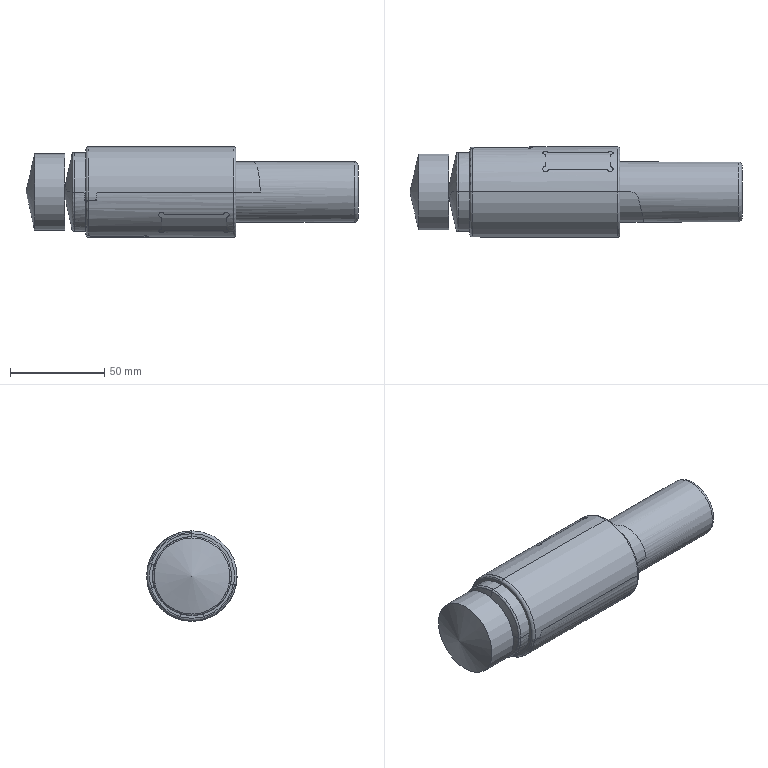NC program | NX | posted with a generic post | part box 176.413 x 48 x 48 mm
Lines 1 to 831 of 2239:
N10 G17 G21 G94 G90
(ZLEVEL_PROFILE_COPY_2_COPY_1 , TOOL : D2)
N12 T02 M6
N14 G54
N16 G17 G0 G90 X-140.296 Y-24.032 S5000 M3
N18 G43 Z25.445 H2
N20 Z1.45
N22 G94 G1 Z-0.05 F1200.
N24 X-140.195 Y-24.058
N26 G3 X-140.002 Y-24.004 R0.2
N28 G1 X-139.927 Y-23.927
N30 X-139.208 Y-23.265
N32 X-132.968 Y-17.507
N34 G2 X-132.658 Y-17.311 R0.846
N36 G3 X-132.419 Y-17.204 R1.166
N38 G1 X-132.394 Y-17.195
N40 X-132.392 Y-17.168
N42 G3 X-134.08 Y-13.44 R3.266
N44 G1 X-134.104 Y-13.434
N46 G3 X-134.442 Y-13.464 R1.291
N48 G2 X-134.903 Y-13.431 R0.896
N50 G1 X-143.562 Y-10.734
N52 G2 X-143.952 Y-10.527 R1.094
N54 G1 X-144.069 Y-10.439
N56 X-144.082 Y-10.455
N58 X-144.182 Y-10.4
N60 X-144.196 Y-10.397
N62 G3 X-146.565 Y-13.718 R3.266
N64 G1 X-146.559 Y-13.743
N66 G3 X-146.363 Y-14.021 R1.291
N68 G2 X-146.161 Y-14.436 R0.892
N70 G1 X-144.732 Y-20.78
N72 X-144.502 Y-21.801
N74 X-144.497 Y-21.83
N76 X-144.489 Y-21.828 Z-0.1
N78 X-144.502 Y-21.761
N80 X-144.723 Y-20.779
N82 X-146.149 Y-14.449
N84 G3 X-146.363 Y-14.021 R0.926
N86 G2 X-146.559 Y-13.743 R1.291
N88 G1 X-146.565 Y-13.718
N90 G2 X-144.196 Y-10.397 R3.266
N92 G1 X-144.182 Y-10.4
N94 X-144.082 Y-10.455
N96 X-144.069 Y-10.439
N98 X-143.998 Y-10.477
N100 X-143.943 Y-10.535
N102 G3 X-143.535 Y-10.752 R1.118
N104 G1 X-134.921 Y-13.435
N106 G3 X-134.442 Y-13.464 R0.929
N108 G2 X-134.104 Y-13.434 R1.291
N110 G1 X-134.08 Y-13.44
N112 G2 X-132.392 Y-17.168 R3.266
N114 G1 X-132.394 Y-17.195
N116 X-132.419 Y-17.204
N118 G2 X-132.668 Y-17.314 R1.166
N120 G3 X-132.989 Y-17.514 R1.087
N122 G1 X-139.221 Y-23.264
N124 X-139.938 Y-23.926
N126 X-140.015 Y-24.003
N128 X-140.027 Z-0.15
N130 X-139.951 Y-23.926
N132 X-139.233 Y-23.264
N134 X-133.009 Y-17.521
N136 G2 X-132.668 Y-17.314 R1.066
N138 G3 X-132.419 Y-17.204 R1.166
N140 G1 X-132.394 Y-17.195
N142 X-132.392 Y-17.168
N144 G3 X-134.08 Y-13.44 R3.266
N146 G1 X-134.104 Y-13.434
N148 G3 X-134.465 Y-13.469 R1.291
N150 G2 X-134.954 Y-13.434 R1.055
N152 G1 X-143.567 Y-10.751
N154 G2 X-143.935 Y-10.542 R1.07
N156 G1 X-143.994 Y-10.48
N158 X-144.069 Y-10.439
N160 X-144.082 Y-10.455
N162 X-144.182 Y-10.4
N164 X-144.196 Y-10.397
N166 G3 X-146.565 Y-13.718 R3.266
N168 G1 X-146.559 Y-13.743
N170 G3 X-146.346 Y-14.039 R1.291
N172 G2 X-146.138 Y-14.463 R1.05
N174 G1 X-144.714 Y-20.779
N176 X-144.496 Y-21.747
N178 X-144.481 Y-21.827
N180 X-144.472 Y-21.826 Z-0.2
N182 X-144.487 Y-21.747
N184 X-144.705 Y-20.779
N186 X-146.126 Y-14.476
N188 G3 X-146.336 Y-14.05 R1.066
N190 G2 X-146.559 Y-13.743 R1.291
N192 G1 X-146.565 Y-13.718
N194 G2 X-144.196 Y-10.397 R3.266
N196 G1 X-144.182 Y-10.4
N198 X-144.082 Y-10.455
N200 X-144.069 Y-10.439
N202 X-143.989 Y-10.484
N204 X-143.926 Y-10.55
N206 G3 X-143.559 Y-10.762 R1.05
N208 G1 X-143.45 Y-10.796
N210 X-134.956 Y-13.442
N212 G3 X-134.476 Y-13.472 R1.065
N214 G2 X-134.104 Y-13.434 R1.291
N216 G1 X-134.08 Y-13.44
N218 G2 X-132.392 Y-17.168 R3.266
N220 G1 X-132.394 Y-17.195
N222 X-132.419 Y-17.204
N224 G2 X-132.686 Y-17.319 R1.166
N226 G3 X-133.029 Y-17.527 R1.086
N228 G1 X-139.246 Y-23.264
N230 X-139.964 Y-23.926
N232 X-140.04 Y-24.001
N234 X-140.053 Y-24. Z-0.25
N236 X-139.977 Y-23.926
N238 X-139.258 Y-23.263
N240 X-133.049 Y-17.534
N242 G2 X-132.696 Y-17.322 R1.072
N244 G3 X-132.419 Y-17.204 R1.166
N246 G1 X-132.394 Y-17.195
N248 X-132.392 Y-17.168
N250 G3 X-134.08 Y-13.44 R3.266
N252 G1 X-134.104 Y-13.434
N254 G3 X-134.476 Y-13.472 R1.291
N256 G2 X-134.972 Y-13.446 R1.043
N258 G1 X-143.453 Y-10.805
N260 G2 X-143.918 Y-10.557 R1.192
N262 G1 X-143.985 Y-10.487
N264 X-144.069 Y-10.439
N266 X-144.082 Y-10.455
N268 X-144.182 Y-10.4
N270 X-144.196 Y-10.397
N272 G3 X-146.565 Y-13.718 R3.266
N274 G1 X-146.559 Y-13.743
N276 G3 X-146.336 Y-14.05 R1.291
N278 G2 X-146.114 Y-14.489 R1.042
N280 G1 X-144.697 Y-20.778
N282 X-144.478 Y-21.747
N284 X-144.464 Y-21.824
N286 X-144.455 Y-21.823 Z-0.3
N288 X-144.469 Y-21.747
N290 X-144.688 Y-20.778
N292 X-146.102 Y-14.501
N294 G3 X-146.336 Y-14.05 R1.03
N296 G2 X-146.559 Y-13.743 R1.291
N298 G1 X-146.565 Y-13.718
N300 G2 X-144.196 Y-10.397 R3.266
N302 G1 X-144.082 Y-10.455
N304 X-144.069 Y-10.439
N306 G2 X-143.91 Y-10.565 R1.166
N308 G3 X-143.456 Y-10.813 R1.15
N310 G1 X-134.989 Y-13.45
N312 G3 X-134.476 Y-13.472 R1.027
N314 G2 X-134.104 Y-13.434 R1.291
N316 G1 X-134.08 Y-13.44
N318 G2 X-132.392 Y-17.168 R3.266
N320 G1 X-132.394 Y-17.195
N322 X-132.419 Y-17.204
N324 G2 X-132.706 Y-17.325 R1.166
N326 G3 X-133.067 Y-17.539 R1.087
N328 G1 X-139.271 Y-23.263
N330 X-139.99 Y-23.926
N332 X-140.066 Y-23.999
N334 X-140.078 Z-0.35
N336 X-140.002 Y-23.926
N338 X-139.283 Y-23.263
N340 X-133.086 Y-17.544
N342 G2 X-132.719 Y-17.328 R1.113
N344 G3 X-132.419 Y-17.204 R1.166
N346 G1 X-132.394 Y-17.195
N348 X-132.392 Y-17.168
N350 G3 X-134.08 Y-13.44 R3.266
N352 G1 X-134.104 Y-13.434
N354 G3 X-134.476 Y-13.472 R1.291
N356 G2 X-135.005 Y-13.454 R0.976
N358 G1 X-143.363 Y-10.851
N360 X-143.507 Y-10.806
N362 G2 X-143.903 Y-10.572 R1.048
N364 G3 X-144.069 Y-10.439 R1.166
N366 G1 X-144.082 Y-10.455
N368 X-144.196 Y-10.397
N370 G3 X-146.565 Y-13.718 R3.266
N372 G1 X-146.559 Y-13.743
N374 G3 X-146.336 Y-14.05 R1.291
N376 G2 X-146.091 Y-14.513 R0.961
N378 G1 X-144.679 Y-20.777
N380 X-144.46 Y-21.747
N382 X-144.447 Y-21.821
N384 X-144.438 Y-21.82 Z-0.4
N386 X-144.451 Y-21.747
N388 X-144.67 Y-20.776
N390 X-146.079 Y-14.526
N392 G3 X-146.336 Y-14.05 R0.991
N394 G2 X-146.559 Y-13.743 R1.291
N396 G1 X-146.565 Y-13.718
N398 G2 X-144.196 Y-10.397 R3.266
N400 G1 X-144.082 Y-10.455
N402 X-144.069 Y-10.439
N404 G2 X-143.895 Y-10.579 R1.166
N406 G3 X-143.461 Y-10.829 R1.071
N408 G1 X-135.022 Y-13.458
N410 G3 X-134.479 Y-13.472 R1.
N412 G2 X-134.104 Y-13.434 R1.291
N414 G1 X-134.08 Y-13.44
N416 G2 X-132.392 Y-17.168 R3.266
N418 G1 X-132.394 Y-17.195
N420 X-132.419 Y-17.204
N422 G2 X-132.733 Y-17.332 R1.166
N424 G3 X-133.105 Y-17.55 R1.129
N426 G1 X-139.294 Y-23.261
N428 X-140.015 Y-23.926
N430 X-140.091 Y-23.998
N432 X-140.103 Y-23.997 Z-0.45
N434 X-140.028 Y-23.926
N436 X-139.306 Y-23.26
N438 X-133.123 Y-17.555
N440 G2 X-132.733 Y-17.332 R1.044
N442 G3 X-132.419 Y-17.204 R1.166
N444 G1 X-132.394 Y-17.195
N446 X-132.392 Y-17.168
N448 G3 X-134.08 Y-13.44 R3.266
N450 G1 X-134.104 Y-13.434
N452 G3 X-134.487 Y-13.475 R1.291
N454 G2 X-135.038 Y-13.462 R1.
N456 G1 X-143.464 Y-10.838
N458 G2 X-143.888 Y-10.586 R1.034
N460 G3 X-144.069 Y-10.439 R1.166
N462 G1 X-144.082 Y-10.455
N464 X-144.196 Y-10.397
N466 G3 X-146.565 Y-13.718 R3.266
N468 G1 X-146.559 Y-13.743
N470 G3 X-146.332 Y-14.054 R1.291
N472 G2 X-146.067 Y-14.537 R1.
N474 G1 X-144.662 Y-20.775
N476 X-144.443 Y-21.747
N478 X-144.43 Y-21.819
N480 X-144.421 Y-21.817 Z-0.5
N482 X-144.434 Y-21.747
N484 X-144.653 Y-20.774
N486 X-146.056 Y-14.548
N488 G3 X-146.325 Y-14.061 R1.
N490 G2 X-146.559 Y-13.743 R1.291
N492 G1 X-146.565 Y-13.718
N494 G2 X-144.196 Y-10.397 R3.266
N496 G1 X-144.082 Y-10.455
N498 X-144.069 Y-10.439
N500 G2 X-143.881 Y-10.594 R1.166
N502 G3 X-143.466 Y-10.846 R1.
N504 G1 X-135.053 Y-13.466
N506 G3 X-134.496 Y-13.477 R1.
N508 G2 X-134.104 Y-13.434 R1.291
N510 G1 X-134.08 Y-13.44
N512 G2 X-132.392 Y-17.168 R3.266
N514 G1 X-132.394 Y-17.195
N516 X-132.419 Y-17.204
N518 G2 X-132.733 Y-17.332 R1.166
N520 G3 X-133.141 Y-17.56 R1.037
N522 G1 X-139.318 Y-23.259
N524 X-140.116 Y-23.996
N526 X-140.128 Y-23.995 Z-0.55
N528 X-139.329 Y-23.258
N530 X-133.159 Y-17.564
N532 G2 X-132.733 Y-17.332 R1.032
N534 G3 X-132.419 Y-17.204 R1.166
N536 G1 X-132.394 Y-17.195
N538 X-132.392 Y-17.168
N540 G3 X-134.08 Y-13.44 R3.266
N542 G1 X-134.104 Y-13.434
N544 G3 X-134.505 Y-13.479 R1.291
N546 G2 X-135.069 Y-13.47 R1.
N548 G1 X-143.109 Y-10.966
N550 X-143.477 Y-10.851
N552 G2 X-143.874 Y-10.6 R1.026
N554 G3 X-144.069 Y-10.439 R1.166
N556 G1 X-144.083 Y-10.455
N558 X-144.196 Y-10.397
N560 G3 X-146.565 Y-13.718 R3.266
N562 G1 X-146.559 Y-13.743
N564 G3 X-146.319 Y-14.067 R1.291
N566 G2 X-146.045 Y-14.56 R1.
N568 G1 X-144.644 Y-20.772
N570 X-144.425 Y-21.747
N572 X-144.412 Y-21.816
N574 X-144.404 Y-21.814 Z-0.6
N576 X-144.416 Y-21.747
N578 X-144.636 Y-20.771
N580 X-146.033 Y-14.571
N582 G3 X-146.312 Y-14.073 R1.
N584 G2 X-146.559 Y-13.743 R1.291
N586 G1 X-146.565 Y-13.718
N588 G2 X-144.196 Y-10.397 R3.266
N590 G1 X-144.083 Y-10.455
N592 X-144.069 Y-10.439
N594 G2 X-143.866 Y-10.609 R1.166
N596 G3 X-143.456 Y-10.865 R0.973
N598 G1 X-143.109 Y-10.975
N600 X-135.084 Y-13.475
N602 G3 X-134.514 Y-13.482 R1.
N604 G2 X-134.104 Y-13.434 R1.291
N606 G1 X-134.08 Y-13.44
N608 G2 X-132.392 Y-17.168 R3.266
N610 G1 X-132.394 Y-17.195
N612 X-132.419 Y-17.204
N614 G2 X-132.735 Y-17.332 R1.166
N616 G3 X-133.176 Y-17.568 R1.
N618 G1 X-139.341 Y-23.258
N620 X-140.126 Y-23.981
N622 X-140.136 Y-23.993
N624 X-140.145 Y-23.99 Z-0.65
N626 X-140.126 Y-23.969
N628 X-139.353 Y-23.256
N630 X-133.193 Y-17.573
N632 G2 X-132.744 Y-17.335 R1.023
N634 G3 X-132.419 Y-17.204 R1.166
N636 G1 X-132.394 Y-17.195
N638 X-132.392 Y-17.168
N640 G3 X-134.08 Y-13.44 R3.266
N642 G1 X-134.104 Y-13.434
N644 G3 X-134.522 Y-13.484 R1.291
N646 G2 X-135.1 Y-13.479 R1.
N648 G1 X-143.109 Y-10.984
N650 X-143.449 Y-10.875
N652 G2 X-143.86 Y-10.615 R0.971
N654 G3 X-144.069 Y-10.439 R1.166
N656 G1 X-144.083 Y-10.455
N658 X-144.196 Y-10.397
N660 G3 X-146.565 Y-13.718 R3.266
N662 G1 X-146.559 Y-13.743
N664 G3 X-146.306 Y-14.08 R1.291
N666 G2 X-146.022 Y-14.582 R1.031
N668 G1 X-144.627 Y-20.77
N670 X-144.407 Y-21.747
N672 X-144.395 Y-21.813
N674 X-144.387 Y-21.811 Z-0.7
N676 X-144.398 Y-21.747
N678 X-146.01 Y-14.593
N680 G3 X-146.3 Y-14.086 R1.031
N682 G2 X-146.559 Y-13.743 R1.291
N684 G1 X-146.565 Y-13.718
N686 G2 X-144.196 Y-10.397 R3.266
N688 G1 X-144.082 Y-10.454
N690 X-144.071 Y-10.459
N692 X-144.063 Y-10.449
N694 X-144.069 Y-10.439
N696 G2 X-143.854 Y-10.621 R1.166
N698 G3 X-143.459 Y-10.877 R0.947
N700 G1 X-143.109 Y-10.993
N702 X-135.114 Y-13.484
N704 G3 X-134.531 Y-13.487 R1.
N706 G2 X-134.104 Y-13.434 R1.291
N708 G1 X-134.08 Y-13.44
N710 G2 X-132.392 Y-17.168 R3.266
N712 G1 X-132.394 Y-17.195
N714 X-132.419 Y-17.204
N716 G2 X-132.753 Y-17.337 R1.166
N718 G3 X-133.211 Y-17.577 R1.029
N720 G1 X-139.364 Y-23.255
N722 X-140.126 Y-23.957
N724 X-140.154 Y-23.988
N726 X-140.163 Y-23.986 Z-0.75
N728 X-140.126 Y-23.946
N730 X-139.375 Y-23.253
N732 X-133.228 Y-17.581
N734 G2 X-132.762 Y-17.339 R1.036
N736 G3 X-132.419 Y-17.204 R1.166
N738 G1 X-132.394 Y-17.195
N740 X-132.392 Y-17.168
N742 G3 X-134.08 Y-13.44 R3.266
N744 G1 X-134.104 Y-13.434
N746 G3 X-134.539 Y-13.489 R1.291
N748 G2 X-134.957 Y-13.525 R1.066
N750 G1 X-135.04 Y-13.522
N752 X-135.117 Y-13.492
N754 X-143.302 Y-10.943
N756 X-143.507 Y-10.872
N758 G2 X-143.848 Y-10.628 R1.038
N760 G3 X-144.069 Y-10.439 R1.166
N762 G1 X-144.083 Y-10.455
N764 X-144.196 Y-10.397
N766 G3 X-146.565 Y-13.718 R3.266
N768 G1 X-146.559 Y-13.743
N770 G3 X-146.293 Y-14.092 R1.291
N772 G2 X-145.999 Y-14.603 R1.034
N774 G1 X-144.61 Y-20.767
N776 X-144.389 Y-21.747
N778 X-144.378 Y-21.81
N780 X-144.369 Y-21.809 Z-0.8
N782 X-144.38 Y-21.747
N784 X-144.602 Y-20.765
N786 X-145.988 Y-14.614
N788 G3 X-146.287 Y-14.097 R1.037
N790 G2 X-146.559 Y-13.743 R1.291
N792 G1 X-146.565 Y-13.718
N794 G2 X-144.196 Y-10.397 R3.266
N796 G1 X-144.083 Y-10.455
N798 X-144.069 Y-10.439
N800 G2 X-143.842 Y-10.635 R1.166
N802 G3 X-143.507 Y-10.879 R1.055
N804 G1 X-143.301 Y-10.952
N806 X-135.144 Y-13.493
N808 G3 X-134.547 Y-13.492 R1.
N810 G2 X-134.104 Y-13.434 R1.291
N812 G1 X-134.08 Y-13.44
N814 G2 X-132.392 Y-17.168 R3.266
N816 G1 X-132.394 Y-17.195
N818 X-132.419 Y-17.204
N820 G2 X-132.771 Y-17.341 R1.166
N822 G3 X-133.247 Y-17.587 R1.035
N824 G1 X-139.386 Y-23.251
N826 X-140.126 Y-23.934
N828 X-140.173 Y-23.983
N830 X-140.182 Y-23.981 Z-0.85
N832 X-140.13 Y-23.926
N834 X-139.397 Y-23.25
N836 X-133.26 Y-17.587
N838 G2 X-132.78 Y-17.342 R1.032
N840 G3 X-132.419 Y-17.204 R1.166
N842 G1 X-132.394 Y-17.195
N844 X-132.392 Y-17.168
N846 G3 X-134.08 Y-13.44 R3.266
N848 G1 X-134.104 Y-13.434
N850 G3 X-134.555 Y-13.494 R1.291
N852 G2 X-135.121 Y-13.503 R0.972
N854 G1 X-135.355 Y-13.436
N856 X-143.3 Y-10.961
N858 G2 X-143.836 Y-10.642 R1.157
N860 G3 X-144.069 Y-10.439 R1.166
N862 G1 X-144.083 Y-10.455
N864 X-144.196 Y-10.397
N866 G3 X-146.565 Y-13.718 R3.266
N868 G1 X-146.559 Y-13.743
N870 G3 X-146.28 Y-14.103 R1.291
N872 G2 X-145.977 Y-14.624 R1.035
N874 G1 X-144.595 Y-20.757
N876 X-144.371 Y-21.747
N878 X-144.361 Y-21.807
N880 X-144.352 Y-21.806 Z-0.9
N882 X-144.362 Y-21.747
N884 X-144.585 Y-20.76
N886 X-145.965 Y-14.634
N888 G3 X-146.274 Y-14.109 R1.026
N890 G2 X-146.559 Y-13.743 R1.291
N892 G1 X-146.565 Y-13.718
N894 G2 X-144.196 Y-10.397 R3.266
N896 G1 X-144.083 Y-10.455
N898 X-144.069 Y-10.439
N900 G2 X-143.83 Y-10.648 R1.166
N902 G3 X-143.299 Y-10.971 R1.136
N904 G1 X-135.415 Y-13.426
N906 X-135.153 Y-13.508
N908 G3 X-134.564 Y-13.497 R1.015
N910 G2 X-134.104 Y-13.434 R1.291
N912 G1 X-134.08 Y-13.44
N914 G2 X-132.392 Y-17.168 R3.266
N916 G1 X-132.394 Y-17.195
N918 X-132.419 Y-17.204
N920 G2 X-132.789 Y-17.344 R1.166
N922 G3 X-133.277 Y-17.59 R1.028
N924 G1 X-139.408 Y-23.248
N926 X-140.143 Y-23.926
N928 X-140.192 Y-23.977
N930 X-140.202 Y-23.974 Z-0.95
N932 X-140.156 Y-23.926
N934 X-139.419 Y-23.246
N936 X-133.293 Y-17.593
N938 G2 X-132.797 Y-17.346 R1.
N940 G3 X-132.419 Y-17.204 R1.166
N942 G1 X-132.394 Y-17.195
N944 X-132.392 Y-17.168
N946 G3 X-134.08 Y-13.44 R3.266
N948 G1 X-134.104 Y-13.434
N950 G3 X-134.571 Y-13.5 R1.291
N952 G2 X-135.153 Y-13.516 R1.014
N954 G1 X-135.444 Y-13.426
N956 X-143.308 Y-10.977
N958 G2 X-143.507 Y-10.902 R1.834
N960 X-143.826 Y-10.653 R1.075
N962 G3 X-144.069 Y-10.439 R1.166
N964 G1 X-144.083 Y-10.455
N966 X-144.196 Y-10.397
N968 G3 X-146.565 Y-13.718 R3.266
N970 G1 X-146.559 Y-13.743
N972 G3 X-146.268 Y-14.114 R1.291
N974 G2 X-145.954 Y-14.644 R1.012
N976 G1 X-144.576 Y-20.759
N978 X-144.354 Y-21.747
N980 X-144.344 Y-21.804
N982 X-144.335 Y-21.803 Z-1.
N984 X-144.345 Y-21.747
N986 X-144.568 Y-20.756
N988 X-145.943 Y-14.653
N990 G3 X-146.262 Y-14.12 R1.
N992 G2 X-146.559 Y-13.743 R1.291
N994 G1 X-146.565 Y-13.718
N996 G2 X-144.196 Y-10.397 R3.266
N998 G1 X-144.083 Y-10.455
N1000 X-144.069 Y-10.439
N1002 G2 X-143.818 Y-10.662 R1.166
N1004 G3 X-143.507 Y-10.909 R1.057
N1006 X-143.308 Y-10.986 R1.57
N1008 G1 X-135.473 Y-13.426
N1010 X-135.193 Y-13.513
N1012 G3 X-134.58 Y-13.503 R0.99
N1014 G2 X-134.104 Y-13.434 R1.291
N1016 G1 X-134.08 Y-13.44
N1018 G2 X-132.392 Y-17.168 R3.266
N1020 G1 X-132.394 Y-17.195
N1022 X-132.419 Y-17.204
N1024 G2 X-132.806 Y-17.347 R1.166
N1026 G3 X-133.309 Y-17.597 R1.
N1028 G1 X-139.429 Y-23.244
N1030 X-140.169 Y-23.926
N1032 X-140.212 Y-23.971
N1034 X-140.222 Y-23.968 Z-1.05
N1036 X-140.182 Y-23.926
N1038 X-139.44 Y-23.242
N1040 X-133.325 Y-17.6
N1042 G2 X-132.815 Y-17.349 R1.
N1044 G3 X-132.419 Y-17.204 R1.166
N1046 G1 X-132.394 Y-17.195
N1048 X-132.392 Y-17.168
N1050 G3 X-134.08 Y-13.44 R3.266
N1052 G1 X-134.104 Y-13.434
N1054 G3 X-134.587 Y-13.505 R1.291
N1056 G2 X-135.153 Y-13.533 R1.011
N1058 G1 X-135.502 Y-13.426
N1060 X-143.349 Y-10.982
N1062 G2 X-143.607 Y-10.856 R0.941
N1064 X-143.813 Y-10.669 R1.249
N1066 G3 X-144.069 Y-10.439 R1.166
N1068 G1 X-144.083 Y-10.455
N1070 X-144.196 Y-10.397
N1072 G3 X-146.565 Y-13.718 R3.266
N1074 G1 X-146.559 Y-13.743
N1076 G3 X-146.256 Y-14.125 R1.291
N1078 G2 X-145.932 Y-14.663 R1.
N1080 G1 X-144.56 Y-20.753
N1082 X-144.336 Y-21.747
N1084 X-144.326 Y-21.801
N1086 X-144.319 Y-21.8 Z-1.075
N1088 X-144.316 Z-1.1
N1090 X-144.327 Y-21.747
N1092 X-144.551 Y-20.751
N1094 X-145.921 Y-14.672
N1096 G3 X-146.249 Y-14.131 R1.
N1098 G2 X-146.559 Y-13.743 R1.291
N1100 G1 X-146.565 Y-13.718
N1102 G2 X-144.196 Y-10.397 R3.266
N1104 G1 X-144.083 Y-10.455
N1106 X-144.069 Y-10.439
N1108 G2 X-143.807 Y-10.675 R1.166
N1110 G3 X-143.308 Y-11.004 R1.02
N1112 G1 X-135.532 Y-13.426
N1114 X-135.153 Y-13.54
N1116 G3 X-134.595 Y-13.508 R1.01
N1118 G2 X-134.104 Y-13.434 R1.291
N1120 G1 X-134.08 Y-13.44
N1122 G2 X-132.392 Y-17.168 R3.266
N1124 G1 X-132.394 Y-17.195
N1126 X-132.419 Y-17.204
N1128 G2 X-132.823 Y-17.35 R1.166
N1130 G3 X-133.341 Y-17.602 R1.
N1132 G1 X-139.45 Y-23.239
N1134 X-140.194 Y-23.926
N1136 X-140.232 Y-23.964
N1138 X-140.242 Y-23.961 Z-1.15
N1140 X-140.207 Y-23.926
N1142 X-139.46 Y-23.237
N1144 X-133.356 Y-17.604
N1146 G2 X-132.831 Y-17.352 R1.
N1148 G3 X-132.419 Y-17.204 R1.166
N1150 G1 X-132.394 Y-17.195
N1152 X-132.392 Y-17.168
N1154 G3 X-134.08 Y-13.44 R3.266
N1156 G1 X-134.104 Y-13.434
N1158 G3 X-134.602 Y-13.51 R1.291
N1160 G2 X-135.153 Y-13.548 R1.012
N1162 G1 X-135.551 Y-13.43
N1164 X-143.308 Y-11.013
N1166 G2 X-143.802 Y-10.682 R1.017
N1168 G3 X-144.069 Y-10.439 R1.166
N1170 G1 X-144.083 Y-10.455
N1172 X-144.196 Y-10.397
N1174 G3 X-146.565 Y-13.718 R3.266
N1176 G1 X-146.559 Y-13.743
N1178 G3 X-146.243 Y-14.136 R1.291
N1180 G2 X-145.91 Y-14.682 R1.
N1182 G1 X-144.543 Y-20.749
N1184 X-144.307 Y-21.798
N1186 X-144.3 Y-21.795 Z-1.2
N1188 X-144.303 Y-21.775
N1190 X-144.577 Y-20.558
N1192 X-145.899 Y-14.691
N1194 G3 X-146.237 Y-14.141 R1.
N1196 G2 X-146.559 Y-13.743 R1.291
N1198 G1 X-146.565 Y-13.718
N1200 G2 X-144.196 Y-10.397 R3.266
N1202 G1 X-144.083 Y-10.455
N1204 X-144.069 Y-10.439
N1206 G2 X-143.797 Y-10.688 R1.166
N1208 G3 X-143.308 Y-11.022 R1.018
N1210 G1 X-135.551 Y-13.439
N1212 X-135.153 Y-13.556
N1214 G3 X-134.61 Y-13.513 R1.01
N1216 G2 X-134.104 Y-13.434 R1.291
N1218 G1 X-134.08 Y-13.44
N1220 G2 X-132.392 Y-17.168 R3.266
N1222 G1 X-132.394 Y-17.195
N1224 X-132.419 Y-17.204
N1226 G2 X-132.84 Y-17.353 R1.166
N1228 G3 X-133.371 Y-17.607 R1.
N1230 G1 X-139.47 Y-23.235
N1232 X-140.22 Y-23.926
N1234 X-140.252 Y-23.958
N1236 X-140.262 Y-23.955 Z-1.25
N1238 X-140.233 Y-23.926
N1240 X-139.481 Y-23.233
N1242 X-133.386 Y-17.609
N1244 G2 X-132.848 Y-17.354 R1.
N1246 G3 X-132.419 Y-17.204 R1.166
N1248 G1 X-132.394 Y-17.195
N1250 X-132.392 Y-17.168
N1252 G3 X-134.08 Y-13.44 R3.266
N1254 G1 X-134.104 Y-13.434
N1256 G3 X-134.618 Y-13.516 R1.291
N1258 G2 X-135.153 Y-13.564 R1.02
N1260 G1 X-135.551 Y-13.448
N1262 X-143.293 Y-11.036
N1264 G2 X-143.792 Y-10.694 R1.015
N1266 G3 X-144.069 Y-10.439 R1.166
N1268 G1 X-144.083 Y-10.455
N1270 X-144.196 Y-10.397
N1272 G3 X-146.565 Y-13.718 R3.266
N1274 G1 X-146.559 Y-13.743
N1276 G3 X-146.231 Y-14.146 R1.291
N1278 G2 X-145.888 Y-14.7 R1.
N1280 G1 X-144.568 Y-20.558
N1282 X-144.3 Y-21.747
N1284 X-144.293 Y-21.791
N1286 X-144.285 Y-21.787 Z-1.3
N1288 X-144.291 Y-21.747
N1290 X-144.559 Y-20.558
N1292 X-145.877 Y-14.709
N1294 G3 X-146.225 Y-14.151 R1.
N1296 G2 X-146.559 Y-13.743 R1.291
N1298 G1 X-146.565 Y-13.718
N1300 G2 X-144.196 Y-10.397 R3.266
N1302 G1 X-144.083 Y-10.455
N1304 X-144.069 Y-10.439
N1306 G2 X-143.787 Y-10.701 R1.166
N1308 G3 X-143.281 Y-11.049 R1.019
N1310 G1 X-135.352 Y-13.519
N1312 X-135.153 Y-13.571
N1314 G3 X-134.625 Y-13.519 R1.028
N1316 G2 X-134.104 Y-13.434 R1.291
N1318 G1 X-134.08 Y-13.44
N1320 G2 X-132.392 Y-17.168 R3.266
N1322 G1 X-132.394 Y-17.195
N1324 X-132.419 Y-17.204
N1326 G2 X-132.856 Y-17.355 R1.166
N1328 G3 X-133.401 Y-17.611 R1.
N1330 G1 X-139.49 Y-23.23
N1332 X-140.246 Y-23.926
N1334 X-140.272 Y-23.952
N1336 X-140.281 Y-23.949 Z-1.35
N1338 X-140.258 Y-23.926
N1340 X-139.5 Y-23.227
N1342 X-133.416 Y-17.613
N1344 G2 X-132.864 Y-17.356 R1.
N1346 G3 X-132.419 Y-17.204 R1.166
N1348 G1 X-132.394 Y-17.195
N1350 X-132.392 Y-17.168
N1352 G3 X-134.08 Y-13.44 R3.266
N1354 G1 X-134.104 Y-13.434
N1356 G3 X-134.632 Y-13.522 R1.291
N1358 G2 X-135.295 Y-13.545 R1.002
N1360 G1 X-143.283 Y-11.057
N1362 G2 X-143.782 Y-10.708 R1.
N1364 G3 X-144.069 Y-10.439 R1.166
N1366 G1 X-144.083 Y-10.455
N1368 X-144.196 Y-10.397
N1370 G3 X-146.565 Y-13.718 R3.266
N1372 G1 X-146.559 Y-13.743
N1374 G3 X-146.219 Y-14.156 R1.291
N1376 G2 X-145.867 Y-14.717 R1.
N1378 G1 X-144.51 Y-20.736
N1380 X-144.282 Y-21.747
N1382 X-144.277 Y-21.782
N1384 X-144.269 Y-21.778 Z-1.4
N1386 X-144.273 Y-21.747
N1388 X-144.502 Y-20.733
N1390 X-145.856 Y-14.726
N1392 G3 X-146.213 Y-14.161 R1.
N1394 G2 X-146.559 Y-13.743 R1.291
N1396 G1 X-146.565 Y-13.718
N1398 G2 X-144.196 Y-10.397 R3.266
N1400 G1 X-144.083 Y-10.455
N1402 X-144.069 Y-10.439
N1404 G2 X-143.777 Y-10.714 R1.166
N1406 G3 X-143.274 Y-11.069 R1.
N1408 G1 X-135.352 Y-13.537
N1410 G3 X-134.63 Y-13.521 R1.021
N1412 G2 X-134.104 Y-13.434 R1.291
N1414 G1 X-134.08 Y-13.44
N1416 G2 X-132.392 Y-17.168 R3.266
N1418 G1 X-132.394 Y-17.195
N1420 X-132.419 Y-17.204
N1422 G2 X-132.872 Y-17.357 R1.166
N1424 G3 X-133.431 Y-17.615 R1.
N1426 G1 X-139.51 Y-23.224
N1428 X-140.291 Y-23.946
N1430 X-140.301 Y-23.942 Z-1.45
N1432 X-139.519 Y-23.221
N1434 X-133.446 Y-17.617
N1436 G2 X-132.88 Y-17.358 R1.
N1438 G3 X-132.419 Y-17.204 R1.166
N1440 G1 X-132.394 Y-17.195
N1442 X-132.392 Y-17.168
N1444 G3 X-134.08 Y-13.44 R3.266
N1446 G1 X-134.104 Y-13.434
N1448 G3 X-134.641 Y-13.525 R1.291
N1450 G2 X-135.352 Y-13.546 R1.014
N1452 G1 X-143.265 Y-11.081
N1454 G2 X-143.772 Y-10.72 R1.015
N1456 G3 X-144.069 Y-10.439 R1.166
N1458 G1 X-144.083 Y-10.455
N1460 X-144.196 Y-10.397
N1462 G3 X-146.565 Y-13.718 R3.266
N1464 G1 X-146.559 Y-13.743
N1466 G3 X-146.206 Y-14.166 R1.291
N1468 G2 X-145.845 Y-14.734 R1.
N1470 G1 X-144.502 Y-20.695
N1472 X-144.265 Y-21.747
N1474 X-144.261 Y-21.774
N1476 X-144.253 Y-21.769 Z-1.5
N1478 X-144.256 Y-21.747
N1480 X-144.486 Y-20.726
N1482 X-145.834 Y-14.743
N1484 G3 X-146.2 Y-14.17 R1.
N1486 G2 X-146.559 Y-13.743 R1.291
N1488 G1 X-146.565 Y-13.718
N1490 G2 X-144.196 Y-10.397 R3.266
N1492 G1 X-144.083 Y-10.455
N1494 X-144.069 Y-10.439
N1496 G2 X-143.768 Y-10.727 R1.166
N1498 G3 X-143.257 Y-11.093 R1.018
N1500 G1 X-135.352 Y-13.555
N1502 G3 X-134.654 Y-13.53 R1.012
N1504 G2 X-134.104 Y-13.434 R1.291
N1506 G1 X-134.08 Y-13.44
N1508 G2 X-132.392 Y-17.168 R3.266
N1510 G1 X-132.394 Y-17.195
N1512 X-132.419 Y-17.204
N1514 G2 X-132.888 Y-17.359 R1.166
N1516 G3 X-133.46 Y-17.618 R1.
N1518 G1 X-139.529 Y-23.218
N1520 X-140.31 Y-23.939
N1522 X-140.32 Y-23.936 Z-1.55
N1524 X-139.539 Y-23.215
N1526 X-133.474 Y-17.619
N1528 G2 X-132.895 Y-17.36 R1.
N1530 G3 X-132.419 Y-17.204 R1.166
N1532 G1 X-132.394 Y-17.195
N1534 X-132.392 Y-17.168
N1536 G3 X-134.08 Y-13.44 R3.266
N1538 G1 X-134.104 Y-13.434
N1540 G3 X-134.661 Y-13.533 R1.291
N1542 G2 X-135.352 Y-13.564 R1.013
N1544 G1 X-143.249 Y-11.105
N1546 G2 X-143.763 Y-10.733 R1.026
N1548 G3 X-144.069 Y-10.439 R1.166
N1550 G1 X-144.083 Y-10.455
N1552 X-144.196 Y-10.397
N1554 G3 X-146.565 Y-13.718 R3.266
N1556 G1 X-146.559 Y-13.743
N1558 G3 X-146.194 Y-14.175 R1.291
N1560 G2 X-145.823 Y-14.751 R1.
N1562 G1 X-144.478 Y-20.723
N1564 X-144.247 Y-21.747
N1566 X-144.244 Y-21.765
N1568 X-144.236 Y-21.761 Z-1.6
N1570 X-144.238 Y-21.747
N1572 X-144.47 Y-20.719
N1574 X-145.813 Y-14.76
N1576 G3 X-146.188 Y-14.18 R1.
N1578 G2 X-146.559 Y-13.743 R1.291
N1580 G1 X-146.565 Y-13.718
N1582 G2 X-144.196 Y-10.397 R3.266
N1584 G1 X-144.083 Y-10.455
N1586 X-144.069 Y-10.439
N1588 G2 X-143.759 Y-10.739 R1.166
N1590 G3 X-143.24 Y-11.116 R1.03
N1592 G1 X-135.359 Y-13.571
N1594 G3 X-135.162 Y-13.611 R0.983
N1596 X-134.668 Y-13.536 R1.021
N1598 G2 X-134.104 Y-13.434 R1.291
N1600 G1 X-134.08 Y-13.44
N1602 G2 X-132.387 Y-17.15 R3.266
N1604 G1 X-132.401 Y-17.163
N1606 X-132.399 Y-17.185
N1608 X-132.419 Y-17.204
N1610 G2 X-132.903 Y-17.36 R1.166
N1612 G3 X-133.489 Y-17.621 R1.
N1614 G1 X-139.548 Y-23.212
N1616 X-140.329 Y-23.933
N1618 X-140.338 Y-23.929 Z-1.65
N1620 X-139.556 Y-23.208
N1622 X-133.503 Y-17.622
N1624 G2 X-132.911 Y-17.361 R1.
N1626 G3 X-132.419 Y-17.204 R1.166
N1628 G1 X-132.399 Y-17.185
N1630 X-132.401 Y-17.163
N1632 X-132.387 Y-17.15
N1634 G3 X-134.08 Y-13.44 R3.266
N1636 G1 X-134.104 Y-13.434
N1638 G3 X-134.675 Y-13.539 R1.291
N1640 G2 X-135.352 Y-13.582 R1.007
N1642 G1 X-135.551 Y-13.52
N1644 X-143.232 Y-11.128
N1646 G2 X-143.754 Y-10.745 R1.03
N1648 G3 X-144.069 Y-10.439 R1.166
N1650 G1 X-144.083 Y-10.455
N1652 X-144.196 Y-10.397
N1654 G3 X-146.565 Y-13.718 R3.266
N1656 G1 X-146.559 Y-13.743
N1658 G3 X-146.182 Y-14.184 R1.291
N1660 G2 X-145.802 Y-14.767 R1.